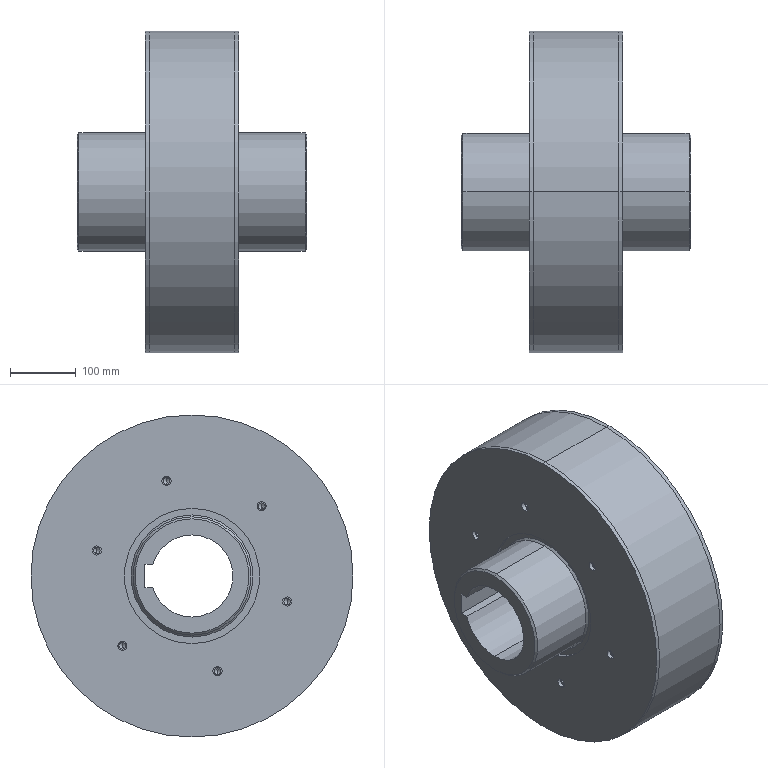Part | SolidWorks | features Chamfer 3, ICE 3, HoleWzd 2, MirrorPattern 2, CirPattern 1, DelFace 1, MirrorSolid 1, MoveFace 1, RevCut 1, Revolution 1, Split 1 | 5 solids | 233 faces | box 350 x 490 x 490 mm | volume 25102965 mm3 | cylinder 147 | cone 44 | torus 24 | plane 18 | commonest cylinder face diameters 40 x55 10.2 x36 14 x24 260 x12 125 x6 490 x6